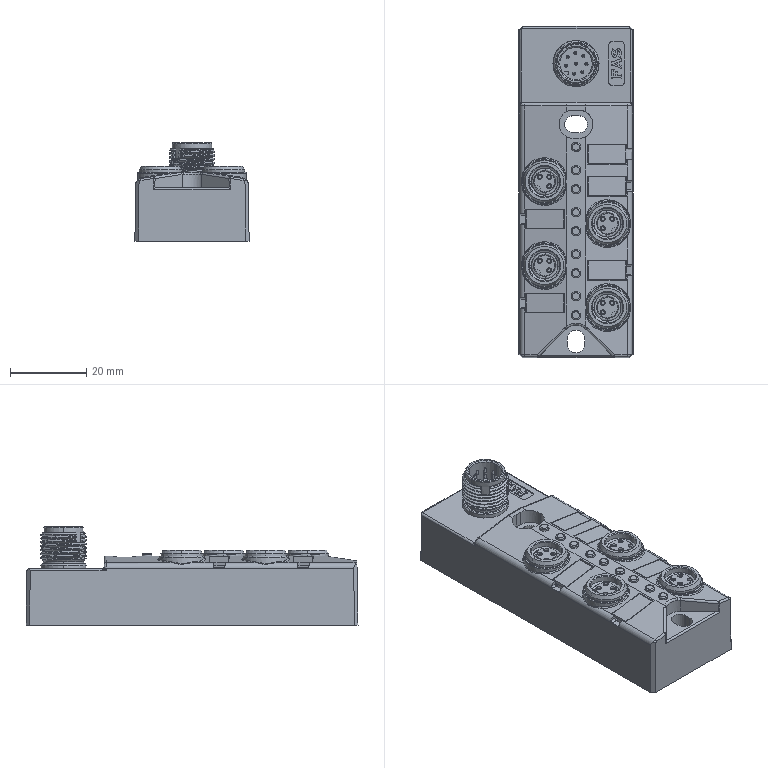Part | STEP file | I/O distribution box 23N4S1 | 3 solids | 2024 faces | box 29.939 x 86.939 x 25.75 mm | volume 38975 mm3 | plane 703 | cylinder 590 | cone 405 | spline 324 | torus 2 | commonest cylinder face diameters 0.8 x106 1.6 x74 1 x60 1.2 x47 8.1 x40 1.35 x36